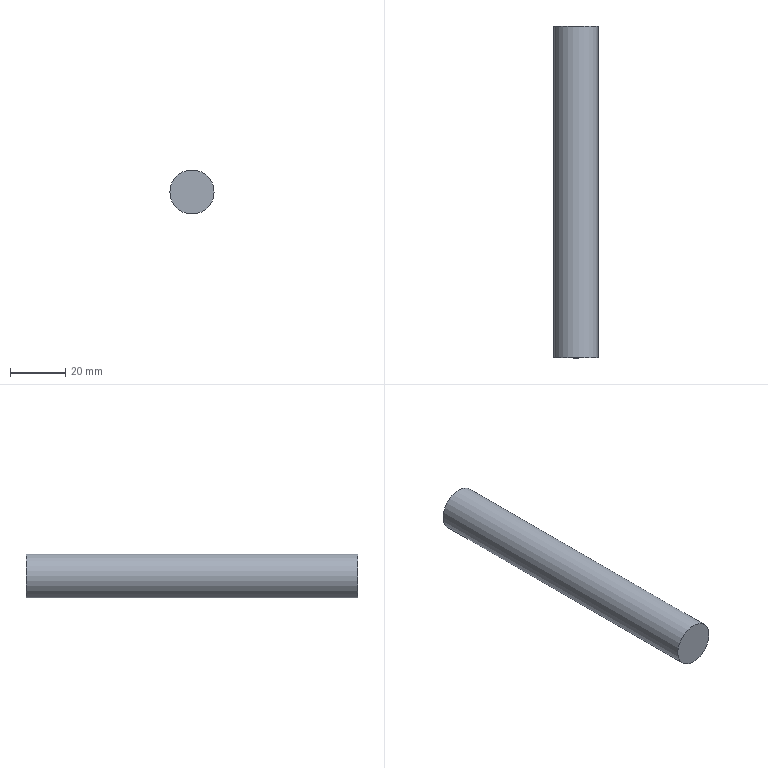Part | STEP file | solid 149 | 1 solid | 3 faces | box 16 x 120 x 16 mm | volume 24127 mm3 | plane 2 | cylinder 1 | commonest cylinder face diameters 16 x1